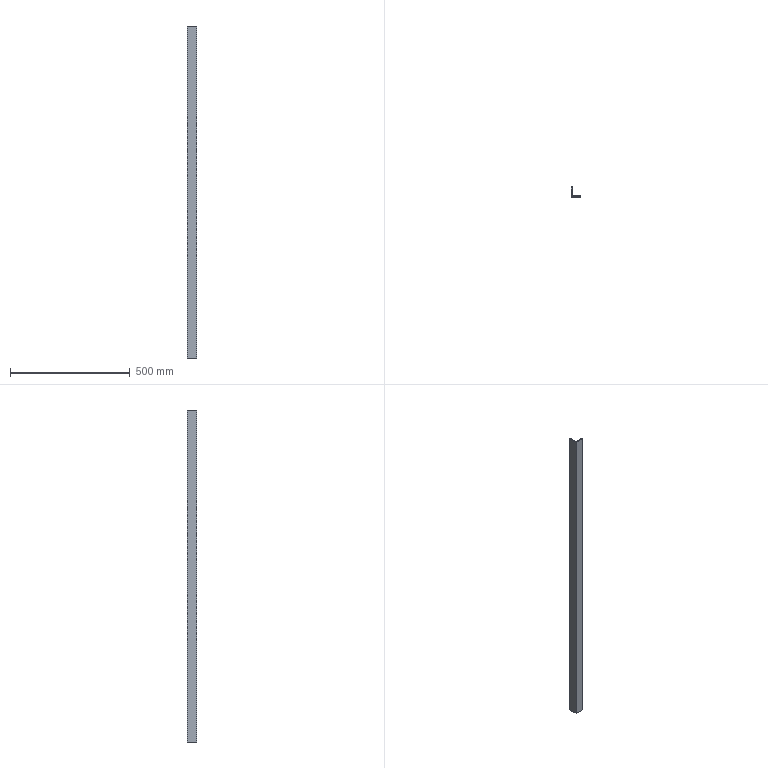Part | SolidWorks | features Extrusion 1 | 1 solid | 11 faces | box 40 x 40 x 1389 mm | volume 428648 mm3 | plane 8 | cylinder 3 | commonest cylinder face diameters 2.667 x2 10 x1
STEP:
#1=CARTESIAN_POINT('',(9.,4.,0.));
#2=VERTEX_POINT('',#1);
#3=CARTESIAN_POINT('',(4.,9.,0.));
#4=VERTEX_POINT('',#3);
#5=CARTESIAN_POINT('',(9.,9.,0.));
#6=DIRECTION('',(0.,0.,-1.));
#7=DIRECTION('',(-1.,0.,0.));
#8=AXIS2_PLACEMENT_3D('',#5,#6,#7);
#9=CIRCLE('',#8,5.);
#10=EDGE_CURVE('',#2,#4,#9,.T.);
#11=ORIENTED_EDGE('',*,*,#10,.T.);
#12=CARTESIAN_POINT('',(4.,9.,1389.));
#13=VERTEX_POINT('',#12);
#14=CARTESIAN_POINT('',(4.,9.,1389.));
#15=DIRECTION('',(0.,0.,-1.));
#16=VECTOR('',#15,1000.);
#17=LINE('',#14,#16);
#18=EDGE_CURVE('',#13,#4,#17,.T.);
#19=ORIENTED_EDGE('',*,*,#18,.F.);
#20=CARTESIAN_POINT('',(9.,4.,1389.));
#21=VERTEX_POINT('',#20);
#22=CARTESIAN_POINT('',(9.,9.,1389.));
#23=DIRECTION('',(0.,0.,-1.));
#24=DIRECTION('',(-1.,0.,0.));
#25=AXIS2_PLACEMENT_3D('',#22,#23,#24);
#26=CIRCLE('',#25,5.);
#27=EDGE_CURVE('',#21,#13,#26,.T.);
#28=ORIENTED_EDGE('',*,*,#27,.F.);
#29=CARTESIAN_POINT('',(9.,4.,1389.));
#30=DIRECTION('',(0.,0.,-1.));
#31=VECTOR('',#30,1000.);
#32=LINE('',#29,#31);
#33=EDGE_CURVE('',#21,#2,#32,.T.);
#34=ORIENTED_EDGE('',*,*,#33,.T.);
#35=EDGE_LOOP('',(#11,#19,#28,#34));
#36=FACE_OUTER_BOUND('',#35,.T.);
#37=CARTESIAN_POINT('',(9.,9.,1389.));
#38=DIRECTION('',(0.,0.,-1.));
#39=DIRECTION('',(-1.,0.,0.));
#40=AXIS2_PLACEMENT_3D('',#37,#38,#39);
#41=CYLINDRICAL_SURFACE('',#40,5.);
#42=ADVANCED_FACE('',(#36),#41,.F.);
#43=CARTESIAN_POINT('',(4.,38.667,0.));
#44=VERTEX_POINT('',#43);
#45=CARTESIAN_POINT('',(4.,38.667,0.));
#46=DIRECTION('',(0.,-1.,0.));
#47=VECTOR('',#46,1000.);
#48=LINE('',#45,#47);
#49=EDGE_CURVE('',#44,#4,#48,.T.);
#50=ORIENTED_EDGE('',*,*,#49,.F.);
#51=CARTESIAN_POINT('',(4.,38.667,1389.));
#52=VERTEX_POINT('',#51);
#53=CARTESIAN_POINT('',(4.,38.667,1389.));
#54=DIRECTION('',(0.,0.,-1.));
#55=VECTOR('',#54,1000.);
#56=LINE('',#53,#55);
#57=EDGE_CURVE('',#52,#44,#56,.T.);
#58=ORIENTED_EDGE('',*,*,#57,.F.);
#59=CARTESIAN_POINT('',(4.,38.667,1389.));
#60=DIRECTION('',(0.,-1.,0.));
#61=VECTOR('',#60,1000.);
#62=LINE('',#59,#61);
#63=EDGE_CURVE('',#52,#13,#62,.T.);
#64=ORIENTED_EDGE('',*,*,#63,.T.);
#65=ORIENTED_EDGE('',*,*,#18,.T.);
#66=EDGE_LOOP('',(#50,#58,#64,#65));
#67=FACE_OUTER_BOUND('',#66,.T.);
#68=CARTESIAN_POINT('',(4.,38.667,1389.));
#69=DIRECTION('',(1.,0.,0.));
#70=DIRECTION('',(0.,1.,0.));
#71=AXIS2_PLACEMENT_3D('',#68,#69,#70);
#72=PLANE('',#71);
#73=ADVANCED_FACE('',(#67),#72,.T.);
#74=CARTESIAN_POINT('',(2.667,40.,0.));
#75=VERTEX_POINT('',#74);
#76=CARTESIAN_POINT('',(2.667,38.667,0.));
#77=DIRECTION('',(0.,0.,-1.));
#78=DIRECTION('',(-1.,0.,0.));
#79=AXIS2_PLACEMENT_3D('',#76,#77,#78);
#80=CIRCLE('',#79,1.333);
#81=EDGE_CURVE('',#75,#44,#80,.T.);
#82=ORIENTED_EDGE('',*,*,#81,.F.);
#83=CARTESIAN_POINT('',(2.667,40.,1389.));
#84=VERTEX_POINT('',#83);
#85=CARTESIAN_POINT('',(2.667,40.,1389.));
#86=DIRECTION('',(0.,0.,-1.));
#87=VECTOR('',#86,1000.);
#88=LINE('',#85,#87);
#89=EDGE_CURVE('',#84,#75,#88,.T.);
#90=ORIENTED_EDGE('',*,*,#89,.F.);
#91=CARTESIAN_POINT('',(2.667,38.667,1389.));
#92=DIRECTION('',(0.,0.,-1.));
#93=DIRECTION('',(-1.,0.,0.));
#94=AXIS2_PLACEMENT_3D('',#91,#92,#93);
#95=CIRCLE('',#94,1.333);
#96=EDGE_CURVE('',#84,#52,#95,.T.);
#97=ORIENTED_EDGE('',*,*,#96,.T.);
#98=ORIENTED_EDGE('',*,*,#57,.T.);
#99=EDGE_LOOP('',(#82,#90,#97,#98));
#100=FACE_OUTER_BOUND('',#99,.T.);
#101=CARTESIAN_POINT('',(2.667,38.667,1389.));
#102=DIRECTION('',(0.,0.,-1.));
#103=DIRECTION('',(-1.,0.,0.));
#104=AXIS2_PLACEMENT_3D('',#101,#102,#103);
#105=CYLINDRICAL_SURFACE('',#104,1.333);
#106=ADVANCED_FACE('',(#100),#105,.T.);
#107=CARTESIAN_POINT('',(0.,40.,0.));
#108=VERTEX_POINT('',#107);
#109=CARTESIAN_POINT('',(0.,40.,0.));
#110=DIRECTION('',(1.,0.,0.));
#111=VECTOR('',#110,1000.);
#112=LINE('',#109,#111);
#113=EDGE_CURVE('',#108,#75,#112,.T.);
#114=ORIENTED_EDGE('',*,*,#113,.F.);
#115=CARTESIAN_POINT('',(0.,40.,1389.));
#116=VERTEX_POINT('',#115);
#117=CARTESIAN_POINT('',(0.,40.,1389.));
#118=DIRECTION('',(0.,0.,-1.));
#119=VECTOR('',#118,1000.);
#120=LINE('',#117,#119);
#121=EDGE_CURVE('',#116,#108,#120,.T.);
#122=ORIENTED_EDGE('',*,*,#121,.F.);
#123=CARTESIAN_POINT('',(0.,40.,1389.));
#124=DIRECTION('',(1.,0.,0.));
#125=VECTOR('',#124,1000.);
#126=LINE('',#123,#125);
#127=EDGE_CURVE('',#116,#84,#126,.T.);
#128=ORIENTED_EDGE('',*,*,#127,.T.);
#129=ORIENTED_EDGE('',*,*,#89,.T.);
#130=EDGE_LOOP('',(#114,#122,#128,#129));
#131=FACE_OUTER_BOUND('',#130,.T.);
#132=CARTESIAN_POINT('',(0.,40.,1389.));
#133=DIRECTION('',(0.,1.,0.));
#134=DIRECTION('',(0.,0.,1.));
#135=AXIS2_PLACEMENT_3D('',#132,#133,#134);
#136=PLANE('',#135);
#137=ADVANCED_FACE('',(#131),#136,.T.);
#138=CARTESIAN_POINT('',(0.,0.,0.));
#139=VERTEX_POINT('',#138);
#140=CARTESIAN_POINT('',(0.,0.,0.));
#141=DIRECTION('',(0.,1.,0.));
#142=VECTOR('',#141,1000.);
#143=LINE('',#140,#142);
#144=EDGE_CURVE('',#139,#108,#143,.T.);
#145=ORIENTED_EDGE('',*,*,#144,.F.);
#146=CARTESIAN_POINT('',(0.,0.,1389.));
#147=VERTEX_POINT('',#146);
#148=CARTESIAN_POINT('',(0.,0.,1389.));
#149=DIRECTION('',(0.,0.,-1.));
#150=VECTOR('',#149,1000.);
#151=LINE('',#148,#150);
#152=EDGE_CURVE('',#147,#139,#151,.T.);
#153=ORIENTED_EDGE('',*,*,#152,.F.);
#154=CARTESIAN_POINT('',(0.,0.,1389.));
#155=DIRECTION('',(0.,1.,0.));
#156=VECTOR('',#155,1000.);
#157=LINE('',#154,#156);
#158=EDGE_CURVE('',#147,#116,#157,.T.);
#159=ORIENTED_EDGE('',*,*,#158,.T.);
#160=ORIENTED_EDGE('',*,*,#121,.T.);
#161=EDGE_LOOP('',(#145,#153,#159,#160));
#162=FACE_OUTER_BOUND('',#161,.T.);
#163=CARTESIAN_POINT('',(0.,0.,1389.));
#164=DIRECTION('',(-1.,0.,0.));
#165=DIRECTION('',(0.,0.,1.));
#166=AXIS2_PLACEMENT_3D('',#163,#164,#165);
#167=PLANE('',#166);
#168=ADVANCED_FACE('',(#162),#167,.T.);
#169=CARTESIAN_POINT('',(40.,0.,0.));
#170=VERTEX_POINT('',#169);
#171=CARTESIAN_POINT('',(40.,0.,0.));
#172=DIRECTION('',(-1.,0.,0.));
#173=VECTOR('',#172,1000.);
#174=LINE('',#171,#173);
#175=EDGE_CURVE('',#170,#139,#174,.T.);
#176=ORIENTED_EDGE('',*,*,#175,.F.);
#177=CARTESIAN_POINT('',(40.,0.,1389.));
#178=VERTEX_POINT('',#177);
#179=CARTESIAN_POINT('',(40.,0.,1389.));
#180=DIRECTION('',(0.,0.,-1.));
#181=VECTOR('',#180,1000.);
#182=LINE('',#179,#181);
#183=EDGE_CURVE('',#178,#170,#182,.T.);
#184=ORIENTED_EDGE('',*,*,#183,.F.);
#185=CARTESIAN_POINT('',(40.,0.,1389.));
#186=DIRECTION('',(-1.,0.,0.));
#187=VECTOR('',#186,1000.);
#188=LINE('',#185,#187);
#189=EDGE_CURVE('',#178,#147,#188,.T.);
#190=ORIENTED_EDGE('',*,*,#189,.T.);
#191=ORIENTED_EDGE('',*,*,#152,.T.);
#192=EDGE_LOOP('',(#176,#184,#190,#191));
#193=FACE_OUTER_BOUND('',#192,.T.);
#194=CARTESIAN_POINT('',(40.,0.,1389.));
#195=DIRECTION('',(0.,-1.,0.));
#196=DIRECTION('',(0.,0.,-1.));
#197=AXIS2_PLACEMENT_3D('',#194,#195,#196);
#198=PLANE('',#197);
#199=ADVANCED_FACE('',(#193),#198,.T.);
#200=CARTESIAN_POINT('',(40.,2.667,0.));
#201=VERTEX_POINT('',#200);
#202=CARTESIAN_POINT('',(40.,0.,0.));
#203=DIRECTION('',(0.,1.,0.));
#204=VECTOR('',#203,1000.);
#205=LINE('',#202,#204);
#206=EDGE_CURVE('',#170,#201,#205,.T.);
#207=ORIENTED_EDGE('',*,*,#206,.T.);
#208=CARTESIAN_POINT('',(40.,2.667,1389.));
#209=VERTEX_POINT('',#208);
#210=CARTESIAN_POINT('',(40.,2.667,1389.));
#211=DIRECTION('',(0.,0.,-1.));
#212=VECTOR('',#211,1000.);
#213=LINE('',#210,#212);
#214=EDGE_CURVE('',#209,#201,#213,.T.);
#215=ORIENTED_EDGE('',*,*,#214,.F.);
#216=CARTESIAN_POINT('',(40.,0.,1389.));
#217=DIRECTION('',(0.,1.,0.));
#218=VECTOR('',#217,1000.);
#219=LINE('',#216,#218);
#220=EDGE_CURVE('',#178,#209,#219,.T.);
#221=ORIENTED_EDGE('',*,*,#220,.F.);
#222=ORIENTED_EDGE('',*,*,#183,.T.);
#223=EDGE_LOOP('',(#207,#215,#221,#222));
#224=FACE_OUTER_BOUND('',#223,.T.);
#225=CARTESIAN_POINT('',(40.,0.,1389.));
#226=DIRECTION('',(-1.,0.,0.));
#227=DIRECTION('',(0.,-1.,0.));
#228=AXIS2_PLACEMENT_3D('',#225,#226,#227);
#229=PLANE('',#228);
#230=ADVANCED_FACE('',(#224),#229,.F.);
#231=CARTESIAN_POINT('',(38.667,4.,0.));
#232=VERTEX_POINT('',#231);
#233=CARTESIAN_POINT('',(38.667,2.667,0.));
#234=DIRECTION('',(0.,0.,1.));
#235=DIRECTION('',(1.,0.,0.));
#236=AXIS2_PLACEMENT_3D('',#233,#234,#235);
#237=CIRCLE('',#236,1.333);
#238=EDGE_CURVE('',#201,#232,#237,.T.);
#239=ORIENTED_EDGE('',*,*,#238,.T.);
#240=CARTESIAN_POINT('',(38.667,4.,1389.));
#241=VERTEX_POINT('',#240);
#242=CARTESIAN_POINT('',(38.667,4.,1389.));
#243=DIRECTION('',(0.,0.,-1.));
#244=VECTOR('',#243,1000.);
#245=LINE('',#242,#244);
#246=EDGE_CURVE('',#241,#232,#245,.T.);
#247=ORIENTED_EDGE('',*,*,#246,.F.);
#248=CARTESIAN_POINT('',(38.667,2.667,1389.));
#249=DIRECTION('',(0.,0.,1.));
#250=DIRECTION('',(1.,0.,0.));
#251=AXIS2_PLACEMENT_3D('',#248,#249,#250);
#252=CIRCLE('',#251,1.333);
#253=EDGE_CURVE('',#209,#241,#252,.T.);
#254=ORIENTED_EDGE('',*,*,#253,.F.);
#255=ORIENTED_EDGE('',*,*,#214,.T.);
#256=EDGE_LOOP('',(#239,#247,#254,#255));
#257=FACE_OUTER_BOUND('',#256,.T.);
#258=CARTESIAN_POINT('',(38.667,2.667,1389.));
#259=DIRECTION('',(0.,0.,-1.));
#260=DIRECTION('',(-1.,0.,0.));
#261=AXIS2_PLACEMENT_3D('',#258,#259,#260);
#262=CYLINDRICAL_SURFACE('',#261,1.333);
#263=ADVANCED_FACE('',(#257),#262,.T.);
#264=CARTESIAN_POINT('',(9.,4.,0.));
#265=DIRECTION('',(1.,0.,0.));
#266=VECTOR('',#265,1000.);
#267=LINE('',#264,#266);
#268=EDGE_CURVE('',#2,#232,#267,.T.);
#269=ORIENTED_EDGE('',*,*,#268,.F.);
#270=ORIENTED_EDGE('',*,*,#33,.F.);
#271=CARTESIAN_POINT('',(9.,4.,1389.));
#272=DIRECTION('',(1.,0.,0.));
#273=VECTOR('',#272,1000.);
#274=LINE('',#271,#273);
#275=EDGE_CURVE('',#21,#241,#274,.T.);
#276=ORIENTED_EDGE('',*,*,#275,.T.);
#277=ORIENTED_EDGE('',*,*,#246,.T.);
#278=EDGE_LOOP('',(#269,#270,#276,#277));
#279=FACE_OUTER_BOUND('',#278,.T.);
#280=CARTESIAN_POINT('',(9.,4.,1389.));
#281=DIRECTION('',(0.,1.,0.));
#282=DIRECTION('',(-1.,0.,0.));
#283=AXIS2_PLACEMENT_3D('',#280,#281,#282);
#284=PLANE('',#283);
#285=ADVANCED_FACE('',(#279),#284,.T.);
#286=ORIENTED_EDGE('',*,*,#27,.T.);
#287=ORIENTED_EDGE('',*,*,#63,.F.);
#288=ORIENTED_EDGE('',*,*,#96,.F.);
#289=ORIENTED_EDGE('',*,*,#127,.F.);
#290=ORIENTED_EDGE('',*,*,#158,.F.);
#291=ORIENTED_EDGE('',*,*,#189,.F.);
#292=ORIENTED_EDGE('',*,*,#220,.T.);
#293=ORIENTED_EDGE('',*,*,#253,.T.);
#294=ORIENTED_EDGE('',*,*,#275,.F.);
#295=EDGE_LOOP('',(#286,#287,#288,#289,#290,#291,#292,#293,#294));
#296=FACE_OUTER_BOUND('',#295,.T.);
#297=CARTESIAN_POINT('',(9.,9.,1389.));
#298=DIRECTION('',(0.,0.,-1.));
#299=DIRECTION('',(-1.,0.,0.));
#300=AXIS2_PLACEMENT_3D('',#297,#298,#299);
#301=PLANE('',#300);
#302=ADVANCED_FACE('',(#296),#301,.F.);
#303=ORIENTED_EDGE('',*,*,#10,.F.);
#304=ORIENTED_EDGE('',*,*,#268,.T.);
#305=ORIENTED_EDGE('',*,*,#238,.F.);
#306=ORIENTED_EDGE('',*,*,#206,.F.);
#307=ORIENTED_EDGE('',*,*,#175,.T.);
#308=ORIENTED_EDGE('',*,*,#144,.T.);
#309=ORIENTED_EDGE('',*,*,#113,.T.);
#310=ORIENTED_EDGE('',*,*,#81,.T.);
#311=ORIENTED_EDGE('',*,*,#49,.T.);
#312=EDGE_LOOP('',(#303,#304,#305,#306,#307,#308,#309,#310,#311));
#313=FACE_OUTER_BOUND('',#312,.T.);
#314=CARTESIAN_POINT('',(9.,9.,0.));
#315=DIRECTION('',(0.,0.,-1.));
#316=DIRECTION('',(-1.,0.,0.));
#317=AXIS2_PLACEMENT_3D('',#314,#315,#316);
#318=PLANE('',#317);
#319=ADVANCED_FACE('',(#313),#318,.T.);
#320=CLOSED_SHELL('',(#42,#73,#106,#137,#168,#199,#230,#263,#285,#302,#319));
#321=MANIFOLD_SOLID_BREP('',#320);
#322=CARTESIAN_POINT('',(0.,0.,0.));
#323=DIRECTION('',(0.,0.,1.));
#324=DIRECTION('',(1.,0.,0.));
#325=AXIS2_PLACEMENT_3D('',#322,#323,#324);
#326=(LENGTH_UNIT()NAMED_UNIT(*)SI_UNIT(.MILLI.,.METRE.));
#327=UNCERTAINTY_MEASURE_WITH_UNIT(LENGTH_MEASURE(0.00001),#326,'','');
#328=(NAMED_UNIT(*)PLANE_ANGLE_UNIT()SI_UNIT($,.RADIAN.));
#329=(NAMED_UNIT(*)SI_UNIT($,.STERADIAN.)SOLID_ANGLE_UNIT());
#330=(GEOMETRIC_REPRESENTATION_CONTEXT(3)GLOBAL_UNCERTAINTY_ASSIGNED_CONTEXT((#327))GLOBAL_UNIT_ASSIGNED_CONTEXT((#326,#328,#329))REPRESENTATION_CONTEXT('',''));
#331=ADVANCED_BREP_SHAPE_REPRESENTATION('',(#321,#325),#330);